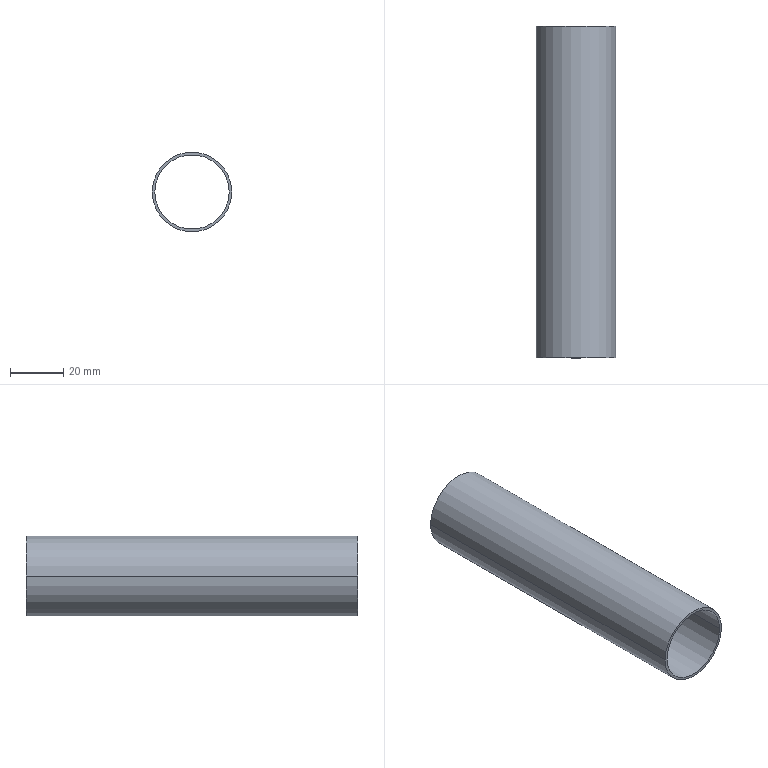Part | STEP file | Component5_1 | 1 solid | 6 faces | box 30 x 125 x 30 mm | volume 11388 mm3 | cylinder 4 | plane 2 | commonest cylinder face diameters 28 x2 30 x2
STEP:
#1=CARTESIAN_POINT('',(1.,140.,17.));
#2=VERTEX_POINT('',#1);
#3=CARTESIAN_POINT('',(29.,140.,17.));
#4=VERTEX_POINT('',#3);
#5=CARTESIAN_POINT('',(15.,140.,17.));
#6=DIRECTION('',(0.,-1.,0.));
#7=DIRECTION('',(1.,0.,0.));
#8=AXIS2_PLACEMENT_3D('',#5,#6,#7);
#9=CIRCLE('',#8,14.);
#10=EDGE_CURVE('',#2,#4,#9,.T.);
#11=ORIENTED_EDGE('',*,*,#10,.F.);
#12=CARTESIAN_POINT('',(1.,15.,17.));
#13=VERTEX_POINT('',#12);
#14=CARTESIAN_POINT('',(1.,140.,17.));
#15=DIRECTION('',(0.,-1.,0.));
#16=VECTOR('',#15,1000.);
#17=LINE('',#14,#16);
#18=EDGE_CURVE('',#2,#13,#17,.T.);
#19=ORIENTED_EDGE('',*,*,#18,.T.);
#20=CARTESIAN_POINT('',(29.,15.,17.));
#21=VERTEX_POINT('',#20);
#22=CARTESIAN_POINT('',(15.,15.,17.));
#23=DIRECTION('',(0.,1.,0.));
#24=DIRECTION('',(1.,0.,0.));
#25=AXIS2_PLACEMENT_3D('',#22,#23,#24);
#26=CIRCLE('',#25,14.);
#27=EDGE_CURVE('',#21,#13,#26,.T.);
#28=ORIENTED_EDGE('',*,*,#27,.F.);
#29=CARTESIAN_POINT('',(29.,140.,17.));
#30=DIRECTION('',(0.,-1.,0.));
#31=VECTOR('',#30,1000.);
#32=LINE('',#29,#31);
#33=EDGE_CURVE('',#4,#21,#32,.T.);
#34=ORIENTED_EDGE('',*,*,#33,.F.);
#35=EDGE_LOOP('',(#11,#19,#28,#34));
#36=FACE_OUTER_BOUND('',#35,.T.);
#37=CARTESIAN_POINT('',(15.,140.,17.));
#38=DIRECTION('',(0.,-1.,0.));
#39=DIRECTION('',(1.,0.,0.));
#40=AXIS2_PLACEMENT_3D('',#37,#38,#39);
#41=CYLINDRICAL_SURFACE('',#40,14.);
#42=ADVANCED_FACE('',(#36),#41,.F.);
#43=CARTESIAN_POINT('',(0.,140.,17.));
#44=VERTEX_POINT('',#43);
#45=CARTESIAN_POINT('',(30.,140.,17.));
#46=VERTEX_POINT('',#45);
#47=CARTESIAN_POINT('',(15.,140.,17.));
#48=DIRECTION('',(0.,1.,0.));
#49=DIRECTION('',(1.,0.,0.));
#50=AXIS2_PLACEMENT_3D('',#47,#48,#49);
#51=CIRCLE('',#50,15.);
#52=EDGE_CURVE('',#44,#46,#51,.T.);
#53=ORIENTED_EDGE('',*,*,#52,.F.);
#54=CARTESIAN_POINT('',(0.,15.,17.));
#55=VERTEX_POINT('',#54);
#56=CARTESIAN_POINT('',(0.,140.,17.));
#57=DIRECTION('',(0.,-1.,0.));
#58=VECTOR('',#57,1000.);
#59=LINE('',#56,#58);
#60=EDGE_CURVE('',#44,#55,#59,.T.);
#61=ORIENTED_EDGE('',*,*,#60,.T.);
#62=CARTESIAN_POINT('',(30.,15.,17.));
#63=VERTEX_POINT('',#62);
#64=CARTESIAN_POINT('',(15.,15.,17.));
#65=DIRECTION('',(0.,-1.,0.));
#66=DIRECTION('',(1.,0.,0.));
#67=AXIS2_PLACEMENT_3D('',#64,#65,#66);
#68=CIRCLE('',#67,15.);
#69=EDGE_CURVE('',#63,#55,#68,.T.);
#70=ORIENTED_EDGE('',*,*,#69,.F.);
#71=CARTESIAN_POINT('',(30.,140.,17.));
#72=DIRECTION('',(0.,-1.,0.));
#73=VECTOR('',#72,1000.);
#74=LINE('',#71,#73);
#75=EDGE_CURVE('',#46,#63,#74,.T.);
#76=ORIENTED_EDGE('',*,*,#75,.F.);
#77=EDGE_LOOP('',(#53,#61,#70,#76));
#78=FACE_OUTER_BOUND('',#77,.T.);
#79=CARTESIAN_POINT('',(15.,140.,17.));
#80=DIRECTION('',(0.,-1.,0.));
#81=DIRECTION('',(1.,0.,0.));
#82=AXIS2_PLACEMENT_3D('',#79,#80,#81);
#83=CYLINDRICAL_SURFACE('',#82,15.);
#84=ADVANCED_FACE('',(#78),#83,.T.);
#85=ORIENTED_EDGE('',*,*,#27,.T.);
#86=CARTESIAN_POINT('',(15.,15.,17.));
#87=DIRECTION('',(0.,1.,0.));
#88=DIRECTION('',(1.,0.,0.));
#89=AXIS2_PLACEMENT_3D('',#86,#87,#88);
#90=CIRCLE('',#89,14.);
#91=EDGE_CURVE('',#13,#21,#90,.T.);
#92=ORIENTED_EDGE('',*,*,#91,.T.);
#93=EDGE_LOOP('',(#85,#92));
#94=FACE_BOUND('',#93,.T.);
#95=ORIENTED_EDGE('',*,*,#69,.T.);
#96=CARTESIAN_POINT('',(15.,15.,17.));
#97=DIRECTION('',(0.,-1.,0.));
#98=DIRECTION('',(1.,0.,0.));
#99=AXIS2_PLACEMENT_3D('',#96,#97,#98);
#100=CIRCLE('',#99,15.);
#101=EDGE_CURVE('',#55,#63,#100,.T.);
#102=ORIENTED_EDGE('',*,*,#101,.T.);
#103=EDGE_LOOP('',(#95,#102));
#104=FACE_OUTER_BOUND('',#103,.T.);
#105=CARTESIAN_POINT('',(15.,15.,17.));
#106=DIRECTION('',(0.,1.,0.));
#107=DIRECTION('',(1.,0.,0.));
#108=AXIS2_PLACEMENT_3D('',#105,#106,#107);
#109=PLANE('',#108);
#110=ADVANCED_FACE('',(#94,#104),#109,.F.);
#111=CARTESIAN_POINT('',(15.,140.,17.));
#112=DIRECTION('',(0.,-1.,0.));
#113=DIRECTION('',(1.,0.,0.));
#114=AXIS2_PLACEMENT_3D('',#111,#112,#113);
#115=CIRCLE('',#114,14.);
#116=EDGE_CURVE('',#4,#2,#115,.T.);
#117=ORIENTED_EDGE('',*,*,#116,.T.);
#118=ORIENTED_EDGE('',*,*,#10,.T.);
#119=EDGE_LOOP('',(#117,#118));
#120=FACE_BOUND('',#119,.T.);
#121=CARTESIAN_POINT('',(15.,140.,17.));
#122=DIRECTION('',(0.,1.,0.));
#123=DIRECTION('',(1.,0.,0.));
#124=AXIS2_PLACEMENT_3D('',#121,#122,#123);
#125=CIRCLE('',#124,15.);
#126=EDGE_CURVE('',#46,#44,#125,.T.);
#127=ORIENTED_EDGE('',*,*,#126,.T.);
#128=ORIENTED_EDGE('',*,*,#52,.T.);
#129=EDGE_LOOP('',(#127,#128));
#130=FACE_OUTER_BOUND('',#129,.T.);
#131=CARTESIAN_POINT('',(15.,140.,17.));
#132=DIRECTION('',(0.,1.,0.));
#133=DIRECTION('',(1.,0.,0.));
#134=AXIS2_PLACEMENT_3D('',#131,#132,#133);
#135=PLANE('',#134);
#136=ADVANCED_FACE('',(#120,#130),#135,.T.);
#137=ORIENTED_EDGE('',*,*,#60,.F.);
#138=ORIENTED_EDGE('',*,*,#126,.F.);
#139=ORIENTED_EDGE('',*,*,#75,.T.);
#140=ORIENTED_EDGE('',*,*,#101,.F.);
#141=EDGE_LOOP('',(#137,#138,#139,#140));
#142=FACE_OUTER_BOUND('',#141,.T.);
#143=CARTESIAN_POINT('',(15.,140.,17.));
#144=DIRECTION('',(0.,-1.,0.));
#145=DIRECTION('',(1.,0.,0.));
#146=AXIS2_PLACEMENT_3D('',#143,#144,#145);
#147=CYLINDRICAL_SURFACE('',#146,15.);
#148=ADVANCED_FACE('',(#142),#147,.T.);
#149=ORIENTED_EDGE('',*,*,#18,.F.);
#150=ORIENTED_EDGE('',*,*,#116,.F.);
#151=ORIENTED_EDGE('',*,*,#33,.T.);
#152=ORIENTED_EDGE('',*,*,#91,.F.);
#153=EDGE_LOOP('',(#149,#150,#151,#152));
#154=FACE_OUTER_BOUND('',#153,.T.);
#155=CARTESIAN_POINT('',(15.,140.,17.));
#156=DIRECTION('',(0.,-1.,0.));
#157=DIRECTION('',(1.,0.,0.));
#158=AXIS2_PLACEMENT_3D('',#155,#156,#157);
#159=CYLINDRICAL_SURFACE('',#158,14.);
#160=ADVANCED_FACE('',(#154),#159,.F.);
#161=CLOSED_SHELL('',(#42,#84,#110,#136,#148,#160));
#162=MANIFOLD_SOLID_BREP('',#161);
#163=CARTESIAN_POINT('',(0.,0.,0.));
#164=DIRECTION('',(0.,0.,1.));
#165=DIRECTION('',(1.,0.,0.));
#166=AXIS2_PLACEMENT_3D('',#163,#164,#165);
#167=(LENGTH_UNIT()NAMED_UNIT(*)SI_UNIT(.MILLI.,.METRE.));
#168=UNCERTAINTY_MEASURE_WITH_UNIT(LENGTH_MEASURE(0.00001),#167,'','');
#169=(NAMED_UNIT(*)PLANE_ANGLE_UNIT()SI_UNIT($,.RADIAN.));
#170=(NAMED_UNIT(*)SI_UNIT($,.STERADIAN.)SOLID_ANGLE_UNIT());
#171=(GEOMETRIC_REPRESENTATION_CONTEXT(3)GLOBAL_UNCERTAINTY_ASSIGNED_CONTEXT((#168))GLOBAL_UNIT_ASSIGNED_CONTEXT((#167,#169,#170))REPRESENTATION_CONTEXT('',''));
#172=ADVANCED_BREP_SHAPE_REPRESENTATION('',(#162,#166),#171);